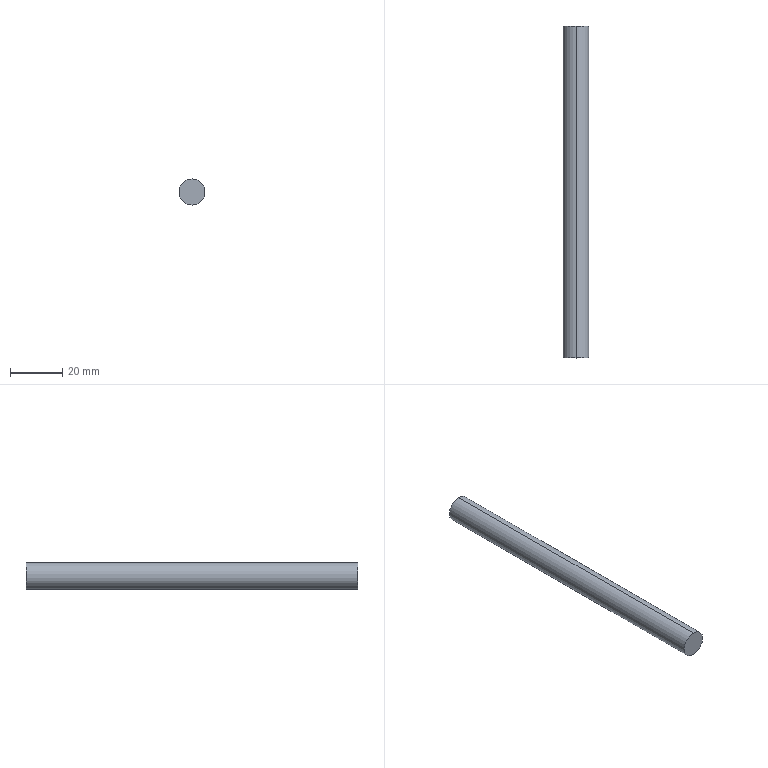Part | 1 solid | 4 faces | box 10 x 127 x 10 mm | volume 9975 mm3 | cylinder 2 | plane 2 | commonest cylinder face diameters 10 x2
STEP:
#1=CARTESIAN_POINT('',(0.,0.,0.));
#2=DIRECTION('',(0.,0.,1.));
#3=DIRECTION('',(1.,0.,0.));
#4=AXIS2_PLACEMENT_3D('',#1,#2,#3);
#5=CARTESIAN_POINT('',(-75.758,69.551,-63.051));
#6=VERTEX_POINT('',#5);
#7=CARTESIAN_POINT('',(-75.758,-57.449,-63.051));
#8=VERTEX_POINT('',#7);
#9=CARTESIAN_POINT('',(-75.758,69.551,-63.051));
#10=DIRECTION('',(0.,-1.,0.));
#11=VECTOR('',#10,1.);
#12=LINE('',#9,#11);
#13=CARTESIAN_POINT('',(-75.758,69.551,-68.051));
#14=DIRECTION('',(0.,-1.,0.));
#15=DIRECTION('',(1.,0.,0.));
#16=AXIS2_PLACEMENT_3D('',#13,#14,#15);
#17=CYLINDRICAL_SURFACE('',#16,5.);
#18=CARTESIAN_POINT('',(1.571,0.));
#19=DIRECTION('',(0.,1.));
#20=VECTOR('',#19,1.);
#21=LINE('',#18,#20);
#22=(GEOMETRIC_REPRESENTATION_CONTEXT(2)PARAMETRIC_REPRESENTATION_CONTEXT()REPRESENTATION_CONTEXT('',''));
#23=DEFINITIONAL_REPRESENTATION('',(#21),#22);
#24=PCURVE('',#17,#23);
#25=CARTESIAN_POINT('',(-75.758,69.551,-68.051));
#26=DIRECTION('',(0.,-1.,0.));
#27=DIRECTION('',(-1.,0.,0.));
#28=AXIS2_PLACEMENT_3D('',#25,#26,#27);
#29=CYLINDRICAL_SURFACE('',#28,5.);
#30=CARTESIAN_POINT('',(4.712,0.));
#31=DIRECTION('',(0.,1.));
#32=VECTOR('',#31,1.);
#33=LINE('',#30,#32);
#34=(GEOMETRIC_REPRESENTATION_CONTEXT(2)PARAMETRIC_REPRESENTATION_CONTEXT()REPRESENTATION_CONTEXT('',''));
#35=DEFINITIONAL_REPRESENTATION('',(#33),#34);
#36=PCURVE('',#29,#35);
#37=SURFACE_CURVE('',#12,(#24,#36),.PCURVE_S1.);
#38=EDGE_CURVE('',#6,#8,#37,.T.);
#39=ORIENTED_EDGE('',*,*,#38,.F.);
#40=CARTESIAN_POINT('',(-75.758,69.551,-73.051));
#41=VERTEX_POINT('',#40);
#42=CARTESIAN_POINT('',(-75.758,69.551,-68.051));
#43=DIRECTION('',(0.,-1.,0.));
#44=DIRECTION('',(0.,0.,-1.));
#45=AXIS2_PLACEMENT_3D('',#42,#43,#44);
#46=CIRCLE('',#45,5.);
#47=CARTESIAN_POINT('',(-1.571,0.));
#48=DIRECTION('',(1.,0.));
#49=VECTOR('',#48,1.);
#50=LINE('',#47,#49);
#51=(GEOMETRIC_REPRESENTATION_CONTEXT(2)PARAMETRIC_REPRESENTATION_CONTEXT()REPRESENTATION_CONTEXT('',''));
#52=DEFINITIONAL_REPRESENTATION('',(#50),#51);
#53=PCURVE('',#17,#52);
#54=CARTESIAN_POINT('',(-75.758,69.551,-68.051));
#55=DIRECTION('',(0.,-1.,0.));
#56=DIRECTION('',(0.,0.,-1.));
#57=AXIS2_PLACEMENT_3D('',#54,#55,#56);
#58=PLANE('',#57);
#59=CARTESIAN_POINT('',(0.,0.));
#60=DIRECTION('',(1.,0.));
#61=AXIS2_PLACEMENT_2D('',#59,#60);
#62=CIRCLE('',#61,5.);
#63=(GEOMETRIC_REPRESENTATION_CONTEXT(2)PARAMETRIC_REPRESENTATION_CONTEXT()REPRESENTATION_CONTEXT('',''));
#64=DEFINITIONAL_REPRESENTATION('',(#62),#63);
#65=PCURVE('',#58,#64);
#66=SURFACE_CURVE('',#46,(#53,#65),.PCURVE_S1.);
#67=EDGE_CURVE('',#6,#41,#66,.T.);
#68=ORIENTED_EDGE('',*,*,#67,.T.);
#69=CARTESIAN_POINT('',(-75.758,-57.449,-73.051));
#70=VERTEX_POINT('',#69);
#71=CARTESIAN_POINT('',(-75.758,69.551,-73.051));
#72=DIRECTION('',(0.,-1.,0.));
#73=VECTOR('',#72,1.);
#74=LINE('',#71,#73);
#75=CARTESIAN_POINT('',(4.712,0.));
#76=DIRECTION('',(0.,1.));
#77=VECTOR('',#76,1.);
#78=LINE('',#75,#77);
#79=(GEOMETRIC_REPRESENTATION_CONTEXT(2)PARAMETRIC_REPRESENTATION_CONTEXT()REPRESENTATION_CONTEXT('',''));
#80=DEFINITIONAL_REPRESENTATION('',(#78),#79);
#81=PCURVE('',#17,#80);
#82=CARTESIAN_POINT('',(1.571,0.));
#83=DIRECTION('',(0.,1.));
#84=VECTOR('',#83,1.);
#85=LINE('',#82,#84);
#86=(GEOMETRIC_REPRESENTATION_CONTEXT(2)PARAMETRIC_REPRESENTATION_CONTEXT()REPRESENTATION_CONTEXT('',''));
#87=DEFINITIONAL_REPRESENTATION('',(#85),#86);
#88=PCURVE('',#29,#87);
#89=SURFACE_CURVE('',#74,(#81,#88),.PCURVE_S1.);
#90=EDGE_CURVE('',#41,#70,#89,.T.);
#91=ORIENTED_EDGE('',*,*,#90,.T.);
#92=CARTESIAN_POINT('',(-75.758,-57.449,-68.051));
#93=DIRECTION('',(0.,-1.,0.));
#94=DIRECTION('',(0.,0.,-1.));
#95=AXIS2_PLACEMENT_3D('',#92,#93,#94);
#96=CIRCLE('',#95,5.);
#97=CARTESIAN_POINT('',(-1.571,127.));
#98=DIRECTION('',(1.,0.));
#99=VECTOR('',#98,1.);
#100=LINE('',#97,#99);
#101=(GEOMETRIC_REPRESENTATION_CONTEXT(2)PARAMETRIC_REPRESENTATION_CONTEXT()REPRESENTATION_CONTEXT('',''));
#102=DEFINITIONAL_REPRESENTATION('',(#100),#101);
#103=PCURVE('',#17,#102);
#104=CARTESIAN_POINT('',(-75.758,-57.449,-68.051));
#105=DIRECTION('',(0.,-1.,0.));
#106=DIRECTION('',(0.,0.,-1.));
#107=AXIS2_PLACEMENT_3D('',#104,#105,#106);
#108=PLANE('',#107);
#109=CARTESIAN_POINT('',(0.,0.));
#110=DIRECTION('',(1.,0.));
#111=AXIS2_PLACEMENT_2D('',#109,#110);
#112=CIRCLE('',#111,5.);
#113=(GEOMETRIC_REPRESENTATION_CONTEXT(2)PARAMETRIC_REPRESENTATION_CONTEXT()REPRESENTATION_CONTEXT('',''));
#114=DEFINITIONAL_REPRESENTATION('',(#112),#113);
#115=PCURVE('',#108,#114);
#116=SURFACE_CURVE('',#96,(#103,#115),.PCURVE_S1.);
#117=EDGE_CURVE('',#8,#70,#116,.T.);
#118=ORIENTED_EDGE('',*,*,#117,.F.);
#119=EDGE_LOOP('',(#39,#68,#91,#118));
#120=FACE_BOUND('',#119,.T.);
#121=ADVANCED_FACE('',(#120),#17,.T.);
#122=ORIENTED_EDGE('',*,*,#67,.F.);
#123=CARTESIAN_POINT('',(-75.758,69.551,-68.051));
#124=DIRECTION('',(0.,-1.,0.));
#125=DIRECTION('',(0.,0.,-1.));
#126=AXIS2_PLACEMENT_3D('',#123,#124,#125);
#127=CIRCLE('',#126,5.);
#128=CARTESIAN_POINT('',(0.,0.));
#129=DIRECTION('',(1.,0.));
#130=AXIS2_PLACEMENT_2D('',#128,#129);
#131=CIRCLE('',#130,5.);
#132=(GEOMETRIC_REPRESENTATION_CONTEXT(2)PARAMETRIC_REPRESENTATION_CONTEXT()REPRESENTATION_CONTEXT('',''));
#133=DEFINITIONAL_REPRESENTATION('',(#131),#132);
#134=PCURVE('',#58,#133);
#135=CARTESIAN_POINT('',(1.571,0.));
#136=DIRECTION('',(1.,0.));
#137=VECTOR('',#136,1.);
#138=LINE('',#135,#137);
#139=(GEOMETRIC_REPRESENTATION_CONTEXT(2)PARAMETRIC_REPRESENTATION_CONTEXT()REPRESENTATION_CONTEXT('',''));
#140=DEFINITIONAL_REPRESENTATION('',(#138),#139);
#141=PCURVE('',#29,#140);
#142=SURFACE_CURVE('',#127,(#134,#141),.PCURVE_S1.);
#143=EDGE_CURVE('',#41,#6,#142,.T.);
#144=ORIENTED_EDGE('',*,*,#143,.F.);
#145=EDGE_LOOP('',(#122,#144));
#146=FACE_BOUND('',#145,.T.);
#147=ADVANCED_FACE('',(#146),#58,.F.);
#148=CARTESIAN_POINT('',(-75.758,-57.449,-68.051));
#149=DIRECTION('',(0.,-1.,0.));
#150=DIRECTION('',(0.,0.,-1.));
#151=AXIS2_PLACEMENT_3D('',#148,#149,#150);
#152=CIRCLE('',#151,5.);
#153=CARTESIAN_POINT('',(0.,0.));
#154=DIRECTION('',(1.,0.));
#155=AXIS2_PLACEMENT_2D('',#153,#154);
#156=CIRCLE('',#155,5.);
#157=(GEOMETRIC_REPRESENTATION_CONTEXT(2)PARAMETRIC_REPRESENTATION_CONTEXT()REPRESENTATION_CONTEXT('',''));
#158=DEFINITIONAL_REPRESENTATION('',(#156),#157);
#159=PCURVE('',#108,#158);
#160=CARTESIAN_POINT('',(1.571,127.));
#161=DIRECTION('',(1.,0.));
#162=VECTOR('',#161,1.);
#163=LINE('',#160,#162);
#164=(GEOMETRIC_REPRESENTATION_CONTEXT(2)PARAMETRIC_REPRESENTATION_CONTEXT()REPRESENTATION_CONTEXT('',''));
#165=DEFINITIONAL_REPRESENTATION('',(#163),#164);
#166=PCURVE('',#29,#165);
#167=SURFACE_CURVE('',#152,(#159,#166),.PCURVE_S1.);
#168=EDGE_CURVE('',#70,#8,#167,.T.);
#169=ORIENTED_EDGE('',*,*,#168,.T.);
#170=ORIENTED_EDGE('',*,*,#117,.T.);
#171=EDGE_LOOP('',(#169,#170));
#172=FACE_BOUND('',#171,.T.);
#173=ADVANCED_FACE('',(#172),#108,.T.);
#174=ORIENTED_EDGE('',*,*,#38,.T.);
#175=ORIENTED_EDGE('',*,*,#168,.F.);
#176=ORIENTED_EDGE('',*,*,#90,.F.);
#177=ORIENTED_EDGE('',*,*,#143,.T.);
#178=EDGE_LOOP('',(#174,#175,#176,#177));
#179=FACE_BOUND('',#178,.T.);
#180=ADVANCED_FACE('',(#179),#29,.T.);
#181=CLOSED_SHELL('',(#121,#147,#173,#180));
#182=MANIFOLD_SOLID_BREP('',#181);
#183=(LENGTH_UNIT()NAMED_UNIT(*)SI_UNIT(.MILLI.,.METRE.));
#184=UNCERTAINTY_MEASURE_WITH_UNIT(LENGTH_MEASURE(0.0000001),#183,'','');
#185=(NAMED_UNIT(*)PLANE_ANGLE_UNIT()SI_UNIT($,.RADIAN.));
#186=(NAMED_UNIT(*)SI_UNIT($,.STERADIAN.)SOLID_ANGLE_UNIT());
#187=(GEOMETRIC_REPRESENTATION_CONTEXT(3)GLOBAL_UNCERTAINTY_ASSIGNED_CONTEXT((#184))GLOBAL_UNIT_ASSIGNED_CONTEXT((#183,#185,#186))REPRESENTATION_CONTEXT('',''));
#188=ADVANCED_BREP_SHAPE_REPRESENTATION('',(#4,#182),#187);